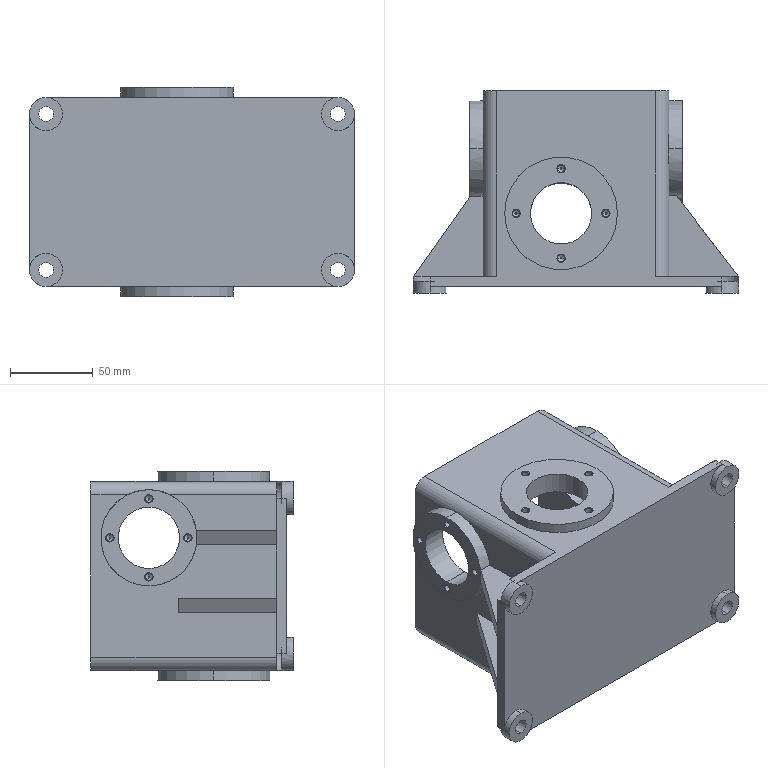Part | SolidWorks | features ICE 13, HoleWzd 5, MirrorPattern 3, Rib 3, DelFace 1, Extrusion 1, Revolution 1 | 1 solid | 257 faces | box 196 x 122 x 126 mm | volume 549396 mm3 | cylinder 105 | cone 96 | plane 52 | sphere 4 | commonest cylinder face diameters 4.2 x48 20 x16 16 x10 9 x8 37 x8 68 x7